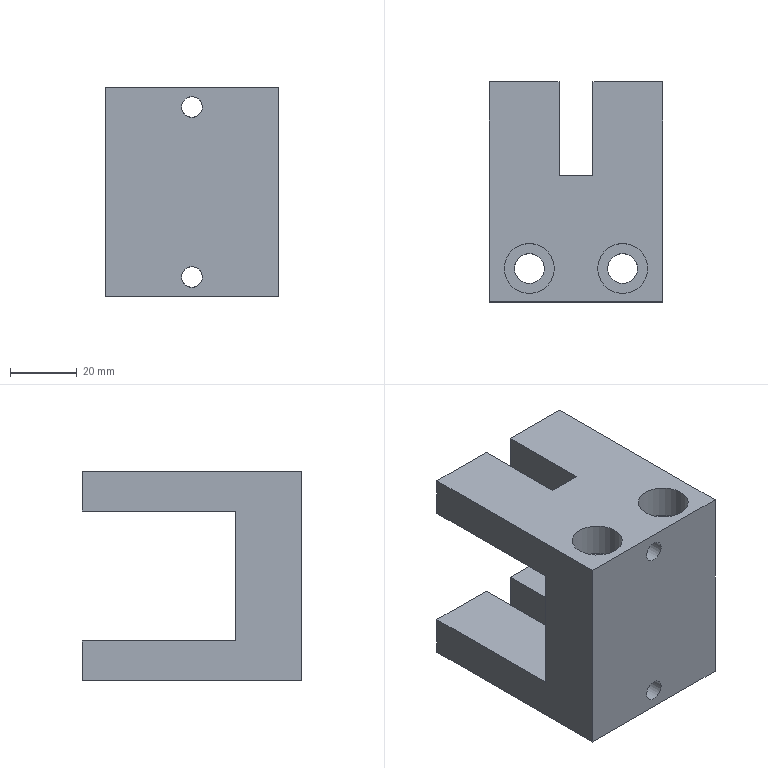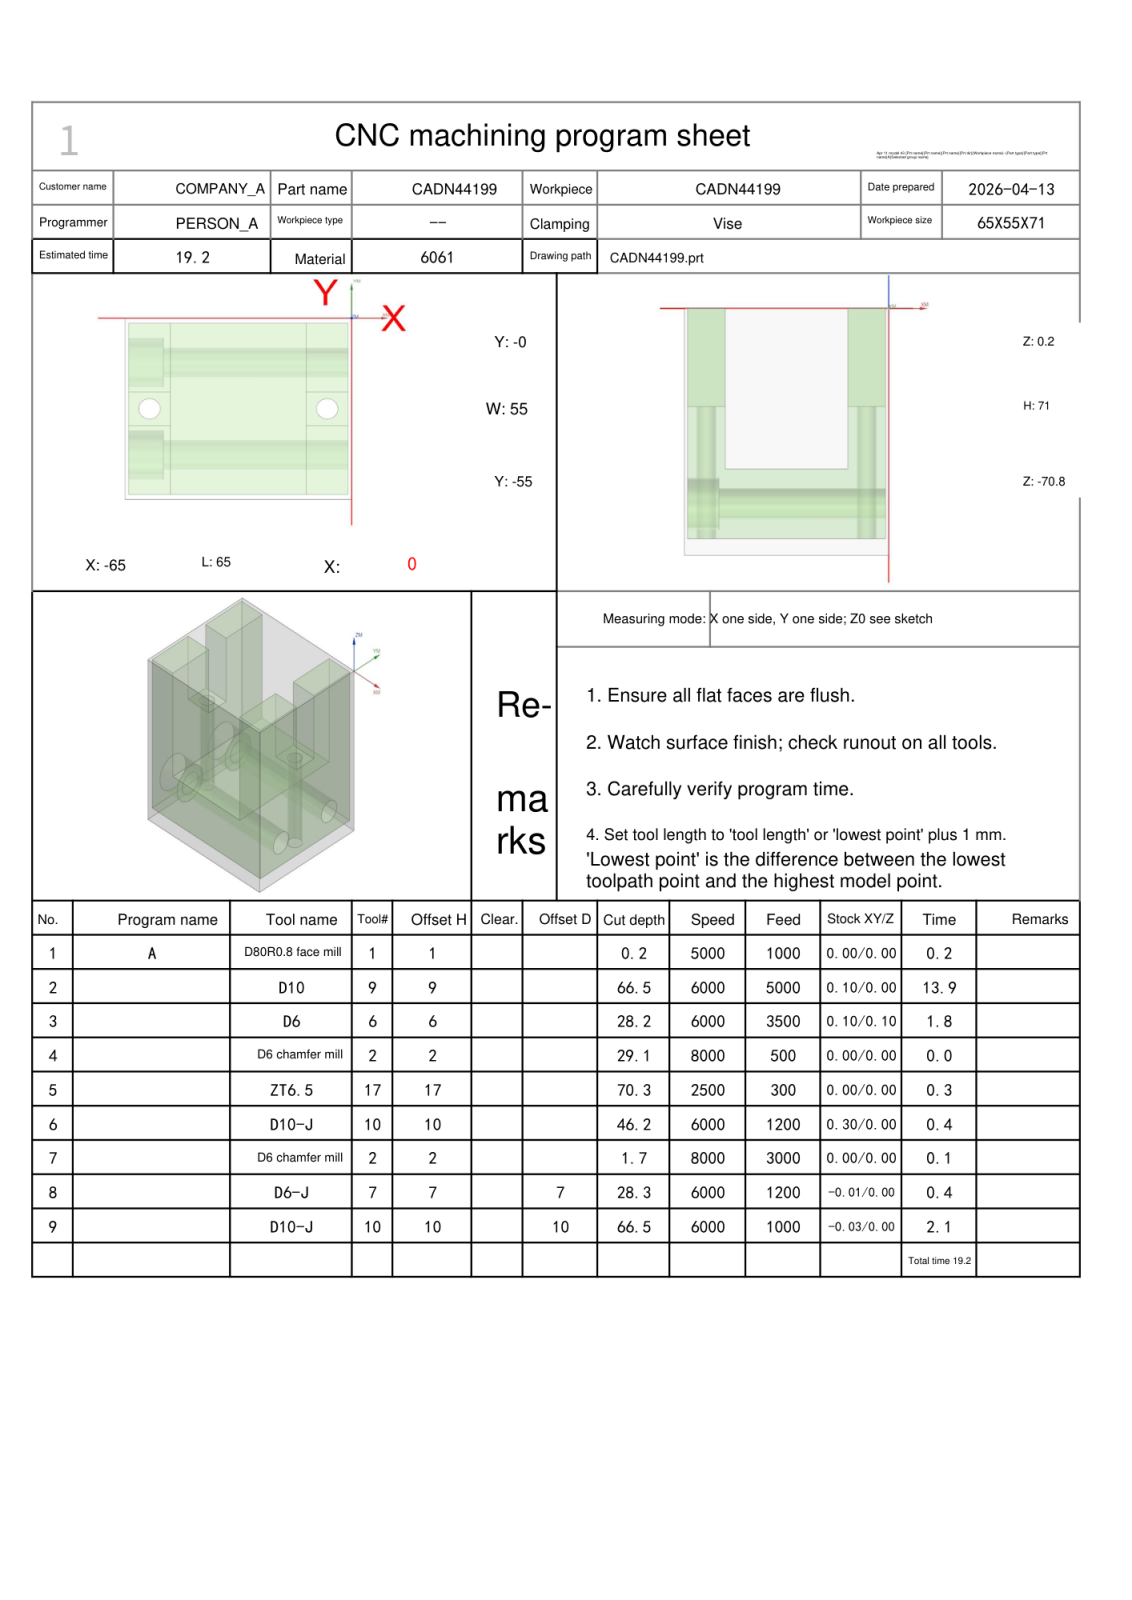NC program | NX | posted by the shop | part box 52 x 66 x 63 mm
Lines 1 to 3030 of 5259, first 2389 of 3028 lines:
%
O0001
(Machine time: 20.73 MIN)
(===Total Tool:7===)
(T1=D80R0.8 face mill D=80.  R=0.8  D-  H01 Z=-0.   )
(T9=D10     D=10.  R=0.   D-  H09 Z=-66.3 )
(T6=D6      D=6.   R=0.   D-  H06 Z=-28.  )
(T2=D6 chamfer mill   D=6.   R=0.   D-  H02 Z=-28.9 )
(T17=ZT6.5  D=6.5  DR_a=118 D-  H17 Z=-70.1 )
(T10=D10-J  D=10.  R=0.   D-  H10 Z=-66.3 )
(T7=D6-J    D=6.   R=0.   D7  H07 Z=-28.1 )
G80 G90 G17 G49 G40
G91 G28 Z0
M01
N1 T01 M06
(D80R0.8 face mill  D=80. R=0.8 H=01 ce=0.00 di=0.00)
G00 G90 G54 X-109. Y-27.5 M03 S5000
G43 H01 Z20.
M08
Z2.
G01 Z0.0 F1000.
X-104.
X39.
X44.
Z2.
G00 Z20.
G91 G28 Z0.0
M05
M09
G91 G28 Z0.0
M01
N2 T09 M06
(D10  D=10. R=0. H=09 ce=0.10 di=0.00)
G00 G90 G54 X-32.5 Y-58.6 M03 S6000
G43 H09 Z20.
M08
Z.5
G01 X-64. Z.404 F5000.
G02 X-69.1 Y-53.5 Z.38 I0.0 J5.1
G01 Y-1.5 Z.222
G02 X-64. Y3.6 Z.198 I5.1 J0.0
G01 X-1. Z.007
G02 X4.1 Y-1.5 Z-.018 I0.0 J-5.1
G01 Y-53.5 Z-.175
G02 X-1. Y-58.6 Z-.2 I-5.1 J0.0
G01 X-64. Z-.391
G02 X-69.1 Y-53.5 Z-.415 I0.0 J5.1
G01 Y-1.5 Z-.573
G02 X-64. Y3.6 Z-.597 I5.1 J0.0
G01 X-1. Z-.788
G02 X4.1 Y-1.5 Z-.813 I0.0 J-5.1
G01 Y-53.5 Z-.971
G02 X-1. Y-58.6 Z-.995 I-5.1 J0.0
G01 X-64. Z-1.186
G02 X-69.1 Y-53.5 Z-1.21 I0.0 J5.1
G01 Y-1.5 Z-1.368
G02 X-64. Y3.6 Z-1.393 I5.1 J0.0
G01 X-1. Z-1.584
G02 X4.1 Y-1.5 Z-1.608 I0.0 J-5.1
G01 Y-53.5 Z-1.766
G02 X-1. Y-58.6 Z-1.79 I-5.1 J0.0
G01 X-64. Z-1.981
G02 X-69.1 Y-53.5 Z-2.006 I0.0 J5.1
G01 Y-1.5 Z-2.163
G02 X-64. Y3.6 Z-2.188 I5.1 J0.0
G01 X-1. Z-2.379
G02 X4.1 Y-1.5 Z-2.403 I0.0 J-5.1
G01 Y-53.5 Z-2.561
G02 X-1. Y-58.6 Z-2.585 I-5.1 J0.0
G01 X-64. Z-2.777
G02 X-69.1 Y-53.5 Z-2.801 I0.0 J5.1
G01 Y-1.5 Z-2.959
G02 X-64. Y3.6 Z-2.983 I5.1 J0.0
G01 X-1. Z-3.174
G02 X4.1 Y-1.5 Z-3.198 I0.0 J-5.1
G01 Y-53.5 Z-3.356
G02 X-1. Y-58.6 Z-3.381 I-5.1 J0.0
G01 X-64. Z-3.572
G02 X-69.1 Y-53.5 Z-3.596 I0.0 J5.1
G01 Y-1.5 Z-3.754
G02 X-64. Y3.6 Z-3.778 I5.1 J0.0
G01 X-1. Z-3.969
G02 X4.1 Y-1.5 Z-3.994 I0.0 J-5.1
G01 Y-53.5 Z-4.152
G02 X-1. Y-58.6 Z-4.176 I-5.1 J0.0
G01 X-64. Z-4.367
G02 X-69.1 Y-53.5 Z-4.391 I0.0 J5.1
G01 Y-1.5 Z-4.549
G02 X-64. Y3.6 Z-4.573 I5.1 J0.0
G01 X-1. Z-4.765
G02 X4.1 Y-1.5 Z-4.789 I0.0 J-5.1
G01 Y-53.5 Z-4.947
G02 X-1. Y-58.6 Z-4.971 I-5.1 J0.0
G01 X-64. Z-5.162
G02 X-69.1 Y-53.5 Z-5.187 I0.0 J5.1
G01 Y-1.5 Z-5.344
G02 X-64. Y3.6 Z-5.369 I5.1 J0.0
G01 X-1. Z-5.56
G02 X4.1 Y-1.5 Z-5.584 I0.0 J-5.1
G01 Y-53.5 Z-5.742
G02 X-1. Y-58.6 Z-5.766 I-5.1 J0.0
G01 X-64. Z-5.958
G02 X-69.1 Y-53.5 Z-5.982 I0.0 J5.1
G01 Y-1.5 Z-6.14
G02 X-64. Y3.6 Z-6.164 I5.1 J0.0
G01 X-1. Z-6.355
G02 X4.1 Y-1.5 Z-6.379 I0.0 J-5.1
G01 Y-53.5 Z-6.537
G02 X-1. Y-58.6 Z-6.562 I-5.1 J0.0
G01 X-64. Z-6.753
G02 X-69.1 Y-53.5 Z-6.777 I0.0 J5.1
G01 Y-1.5 Z-6.935
G02 X-64. Y3.6 Z-6.959 I5.1 J0.0
G01 X-1. Z-7.15
G02 X4.1 Y-1.5 Z-7.175 I0.0 J-5.1
G01 Y-53.5 Z-7.332
G02 X-1. Y-58.6 Z-7.357 I-5.1 J0.0
G01 X-64. Z-7.548
G02 X-69.1 Y-53.5 Z-7.572 I0.0 J5.1
G01 Y-1.5 Z-7.73
G02 X-64. Y3.6 Z-7.754 I5.1 J0.0
G01 X-1. Z-7.946
G02 X4.1 Y-1.5 Z-7.97 I0.0 J-5.1
G01 Y-53.5 Z-8.128
G02 X-1. Y-58.6 Z-8.152 I-5.1 J0.0
G01 X-64. Z-8.343
G02 X-69.1 Y-53.5 Z-8.368 I0.0 J5.1
G01 Y-1.5 Z-8.525
G02 X-64. Y3.6 Z-8.55 I5.1 J0.0
G01 X-1. Z-8.741
G02 X4.1 Y-1.5 Z-8.765 I0.0 J-5.1
G01 Y-53.5 Z-8.923
G02 X-1. Y-58.6 Z-8.947 I-5.1 J0.0
G01 X-64. Z-9.138
G02 X-69.1 Y-53.5 Z-9.163 I0.0 J5.1
G01 Y-1.5 Z-9.321
G02 X-64. Y3.6 Z-9.345 I5.1 J0.0
G01 X-1. Z-9.536
G02 X4.1 Y-1.5 Z-9.56 I0.0 J-5.1
G01 Y-53.5 Z-9.718
G02 X-1. Y-58.6 Z-9.743 I-5.1 J0.0
G01 X-64. Z-9.934
G02 X-69.1 Y-53.5 Z-9.958 I0.0 J5.1
G01 Y-1.5 Z-10.116
G02 X-64. Y3.6 Z-10.14 I5.1 J0.0
G01 X-1. Z-10.331
G02 X4.1 Y-1.5 Z-10.356 I0.0 J-5.1
G01 Y-53.5 Z-10.513
G02 X-1. Y-58.6 Z-10.538 I-5.1 J0.0
G01 X-64. Z-10.729
G02 X-69.1 Y-53.5 Z-10.753 I0.0 J5.1
G01 Y-1.5 Z-10.911
G02 X-64. Y3.6 Z-10.935 I5.1 J0.0
G01 X-1. Z-11.127
G02 X4.1 Y-1.5 Z-11.151 I0.0 J-5.1
G01 Y-53.5 Z-11.309
G02 X-1. Y-58.6 Z-11.333 I-5.1 J0.0
G01 X-64. Z-11.524
G02 X-69.1 Y-53.5 Z-11.548 I0.0 J5.1
G01 Y-1.5 Z-11.706
G02 X-64. Y3.6 Z-11.731 I5.1 J0.0
G01 X-1. Z-11.922
G02 X4.1 Y-1.5 Z-11.946 I0.0 J-5.1
G01 Y-53.5 Z-12.104
G02 X-1. Y-58.6 Z-12.128 I-5.1 J0.0
G01 X-64. Z-12.319
G02 X-69.1 Y-53.5 Z-12.344 I0.0 J5.1
G01 Y-1.5 Z-12.502
G02 X-64. Y3.6 Z-12.526 I5.1 J0.0
G01 X-1. Z-12.717
G02 X4.1 Y-1.5 Z-12.741 I0.0 J-5.1
G01 Y-53.5 Z-12.899
G02 X-1. Y-58.6 Z-12.923 I-5.1 J0.0
G01 X-64. Z-13.115
G02 X-69.1 Y-53.5 Z-13.139 I0.0 J5.1
G01 Y-1.5 Z-13.297
G02 X-64. Y3.6 Z-13.321 I5.1 J0.0
G01 X-1. Z-13.512
G02 X4.1 Y-1.5 Z-13.537 I0.0 J-5.1
G01 Y-53.5 Z-13.694
G02 X-1. Y-58.6 Z-13.719 I-5.1 J0.0
G01 X-64. Z-13.91
G02 X-69.1 Y-53.5 Z-13.934 I0.0 J5.1
G01 Y-1.5 Z-14.092
G02 X-64. Y3.6 Z-14.116 I5.1 J0.0
G01 X-1. Z-14.308
G02 X4.1 Y-1.5 Z-14.332 I0.0 J-5.1
G01 Y-53.5 Z-14.49
G02 X-1. Y-58.6 Z-14.514 I-5.1 J0.0
G01 X-64. Z-14.705
G02 X-69.1 Y-53.5 Z-14.729 I0.0 J5.1
G01 Y-1.5 Z-14.887
G02 X-64. Y3.6 Z-14.912 I5.1 J0.0
G01 X-1. Z-15.103
G02 X4.1 Y-1.5 Z-15.127 I0.0 J-5.1
G01 Y-53.5 Z-15.285
G02 X-1. Y-58.6 Z-15.309 I-5.1 J0.0
G01 X-64. Z-15.5
G02 X-69.1 Y-53.5 Z-15.525 I0.0 J5.1
G01 Y-1.5 Z-15.682
G02 X-64. Y3.6 Z-15.707 I5.1 J0.0
G01 X-1. Z-15.898
G02 X4.1 Y-1.5 Z-15.922 I0.0 J-5.1
G01 Y-53.5 Z-16.08
G02 X-1. Y-58.6 Z-16.104 I-5.1 J0.0
G01 X-64. Z-16.296
G02 X-69.1 Y-53.5 Z-16.32 I0.0 J5.1
G01 Y-1.5 Z-16.478
G02 X-64. Y3.6 Z-16.502 I5.1 J0.0
G01 X-1. Z-16.693
G02 X4.1 Y-1.5 Z-16.718 I0.0 J-5.1
G01 Y-53.5 Z-16.875
G02 X-1. Y-58.6 Z-16.9 I-5.1 J0.0
G01 X-64. Z-17.091
G02 X-69.1 Y-53.5 Z-17.115 I0.0 J5.1
G01 Y-1.5 Z-17.273
G02 X-64. Y3.6 Z-17.297 I5.1 J0.0
G01 X-1. Z-17.488
G02 X4.1 Y-1.5 Z-17.513 I0.0 J-5.1
G01 Y-53.5 Z-17.671
G02 X-1. Y-58.6 Z-17.695 I-5.1 J0.0
G01 X-64. Z-17.886
G02 X-69.1 Y-53.5 Z-17.91 I0.0 J5.1
G01 Y-1.5 Z-18.068
G02 X-64. Y3.6 Z-18.093 I5.1 J0.0
G01 X-1. Z-18.284
G02 X4.1 Y-1.5 Z-18.308 I0.0 J-5.1
G01 Y-53.5 Z-18.466
G02 X-1. Y-58.6 Z-18.49 I-5.1 J0.0
G01 X-64. Z-18.681
G02 X-69.1 Y-53.5 Z-18.706 I0.0 J5.1
G01 Y-1.5 Z-18.863
G02 X-64. Y3.6 Z-18.888 I5.1 J0.0
G01 X-1. Z-19.079
G02 X4.1 Y-1.5 Z-19.103 I0.0 J-5.1
G01 Y-53.5 Z-19.261
G02 X-1. Y-58.6 Z-19.285 I-5.1 J0.0
G01 X-64. Z-19.477
G02 X-69.1 Y-53.5 Z-19.501 I0.0 J5.1
G01 Y-1.5 Z-19.659
G02 X-64. Y3.6 Z-19.683 I5.1 J0.0
G01 X-1. Z-19.874
G02 X4.1 Y-1.5 Z-19.898 I0.0 J-5.1
G01 Y-53.5 Z-20.056
G02 X-1. Y-58.6 Z-20.081 I-5.1 J0.0
G01 X-64. Z-20.272
G02 X-69.1 Y-53.5 Z-20.296 I0.0 J5.1
G01 Y-1.5 Z-20.454
G02 X-64. Y3.6 Z-20.478 I5.1 J0.0
G01 X-1. Z-20.669
G02 X4.1 Y-1.5 Z-20.694 I0.0 J-5.1
G01 Y-53.5 Z-20.852
G02 X-1. Y-58.6 Z-20.876 I-5.1 J0.0
G01 X-64. Z-21.067
G02 X-69.1 Y-53.5 Z-21.091 I0.0 J5.1
G01 Y-1.5 Z-21.249
G02 X-64. Y3.6 Z-21.273 I5.1 J0.0
G01 X-1. Z-21.465
G02 X4.1 Y-1.5 Z-21.489 I0.0 J-5.1
G01 Y-53.5 Z-21.647
G02 X-1. Y-58.6 Z-21.671 I-5.1 J0.0
G01 X-64. Z-21.862
G02 X-69.1 Y-53.5 Z-21.887 I0.0 J5.1
G01 Y-1.5 Z-22.044
G02 X-64. Y3.6 Z-22.069 I5.1 J0.0
G01 X-1. Z-22.26
G02 X4.1 Y-1.5 Z-22.284 I0.0 J-5.1
G01 Y-53.5 Z-22.442
G02 X-1. Y-58.6 Z-22.466 I-5.1 J0.0
G01 X-64. Z-22.658
G02 X-69.1 Y-53.5 Z-22.682 I0.0 J5.1
G01 Y-1.5 Z-22.84
G02 X-64. Y3.6 Z-22.864 I5.1 J0.0
G01 X-1. Z-23.055
G02 X4.1 Y-1.5 Z-23.079 I0.0 J-5.1
G01 Y-53.5 Z-23.237
G02 X-1. Y-58.6 Z-23.262 I-5.1 J0.0
G01 X-64. Z-23.453
G02 X-69.1 Y-53.5 Z-23.477 I0.0 J5.1
G01 Y-1.5 Z-23.635
G02 X-64. Y3.6 Z-23.659 I5.1 J0.0
G01 X-1. Z-23.85
G02 X4.1 Y-1.5 Z-23.875 I0.0 J-5.1
G01 Y-53.5 Z-24.032
G02 X-1. Y-58.6 Z-24.057 I-5.1 J0.0
G01 X-64. Z-24.248
G02 X-69.1 Y-53.5 Z-24.272 I0.0 J5.1
G01 Y-1.5 Z-24.43
G02 X-64. Y3.6 Z-24.454 I5.1 J0.0
G01 X-1. Z-24.646
G02 X4.1 Y-1.5 Z-24.67 I0.0 J-5.1
G01 Y-53.5 Z-24.828
G02 X-1. Y-58.6 Z-24.852 I-5.1 J0.0
G01 X-64. Z-25.043
G02 X-69.1 Y-53.5 Z-25.068 I0.0 J5.1
G01 Y-1.5 Z-25.225
G02 X-64. Y3.6 Z-25.25 I5.1 J0.0
G01 X-1. Z-25.441
G02 X4.1 Y-1.5 Z-25.465 I0.0 J-5.1
G01 Y-53.5 Z-25.623
G02 X-1. Y-58.6 Z-25.647 I-5.1 J0.0
G01 X-64. Z-25.838
G02 X-69.1 Y-53.5 Z-25.863 I0.0 J5.1
G01 Y-1.5 Z-26.021
G02 X-64. Y3.6 Z-26.045 I5.1 J0.0
G01 X-1. Z-26.236
G02 X4.1 Y-1.5 Z-26.26 I0.0 J-5.1
G01 Y-53.5 Z-26.418
G02 X-1. Y-58.6 Z-26.443 I-5.1 J0.0
G01 X-64. Z-26.634
G02 X-69.1 Y-53.5 Z-26.658 I0.0 J5.1
G01 Y-1.5 Z-26.816
G02 X-64. Y3.6 Z-26.84 I5.1 J0.0
G01 X-1. Z-27.031
G02 X4.1 Y-1.5 Z-27.056 I0.0 J-5.1
G01 Y-53.5 Z-27.213
G02 X-1. Y-58.6 Z-27.238 I-5.1 J0.0
G01 X-64. Z-27.429
G02 X-69.1 Y-53.5 Z-27.453 I0.0 J5.1
G01 Y-1.5 Z-27.611
G02 X-64. Y3.6 Z-27.635 I5.1 J0.0
G01 X-1. Z-27.827
G02 X4.1 Y-1.5 Z-27.851 I0.0 J-5.1
G01 Y-53.5 Z-28.009
G02 X-1. Y-58.6 Z-28.033 I-5.1 J0.0
G01 X-64. Z-28.224
G02 X-69.1 Y-53.5 Z-28.248 I0.0 J5.1
G01 Y-1.5 Z-28.406
G02 X-64. Y3.6 Z-28.431 I5.1 J0.0
G01 X-1. Z-28.622
G02 X4.1 Y-1.5 Z-28.646 I0.0 J-5.1
G01 Y-53.5 Z-28.804
G02 X-1. Y-58.6 Z-28.828 I-5.1 J0.0
G01 X-64. Z-29.019
G02 X-69.1 Y-53.5 Z-29.044 I0.0 J5.1
G01 Y-1.5 Z-29.202
G02 X-64. Y3.6 Z-29.226 I5.1 J0.0
G01 X-1. Z-29.417
G02 X4.1 Y-1.5 Z-29.441 I0.0 J-5.1
G01 Y-53.5 Z-29.599
G02 X-1. Y-58.6 Z-29.623 I-5.1 J0.0
G01 X-64. Z-29.815
G02 X-69.1 Y-53.5 Z-29.839 I0.0 J5.1
G01 Y-1.5 Z-29.997
G02 X-64. Y3.6 Z-30.021 I5.1 J0.0
G01 X-1. Z-30.212
G02 X4.1 Y-1.5 Z-30.237 I0.0 J-5.1
G01 Y-53.5 Z-30.394
G02 X-1. Y-58.6 Z-30.419 I-5.1 J0.0
G01 X-64. Z-30.61
G02 X-69.1 Y-53.5 Z-30.634 I0.0 J5.1
G01 Y-1.5 Z-30.792
G02 X-64. Y3.6 Z-30.816 I5.1 J0.0
G01 X-1. Z-31.008
G02 X4.1 Y-1.5 Z-31.032 I0.0 J-5.1
G01 Y-53.5 Z-31.19
G02 X-1. Y-58.6 Z-31.214 I-5.1 J0.0
G01 X-64. Z-31.405
G02 X-69.1 Y-53.5 Z-31.429 I0.0 J5.1
G01 Y-1.5 Z-31.587
G02 X-64. Y3.6 Z-31.612 I5.1 J0.0
G01 X-1. Z-31.803
G02 X4.1 Y-1.5 Z-31.827 I0.0 J-5.1
G01 Y-53.5 Z-31.985
G02 X-1. Y-58.6 Z-32.009 I-5.1 J0.0
G01 X-64. Z-32.2
G02 X-69.1 Y-53.5 Z-32.225 I0.0 J5.1
G01 Y-1.5 Z-32.382
G02 X-64. Y3.6 Z-32.407 I5.1 J0.0
G01 X-1. Z-32.598
G02 X4.1 Y-1.5 Z-32.622 I0.0 J-5.1
G01 Y-53.5 Z-32.78
G02 X-1. Y-58.6 Z-32.804 I-5.1 J0.0
G01 X-64. Z-32.996
G02 X-69.1 Y-53.5 Z-33.02 I0.0 J5.1
G01 Y-1.5 Z-33.178
G02 X-64. Y3.6 Z-33.202 I5.1 J0.0
G01 X-1. Z-33.393
G02 X4.1 Y-1.5 Z-33.418 I0.0 J-5.1
G01 Y-53.5 Z-33.575
G02 X-1. Y-58.6 Z-33.6 I-5.1 J0.0
G01 X-64. Z-33.791
G02 X-69.1 Y-53.5 Z-33.815 I0.0 J5.1
G01 Y-1.5 Z-33.973
G02 X-64. Y3.6 Z-33.997 I5.1 J0.0
G01 X-1. Z-34.188
G02 X4.1 Y-1.5 Z-34.213 I0.0 J-5.1
G01 Y-53.5 Z-34.371
G02 X-1. Y-58.6 Z-34.395 I-5.1 J0.0
G01 X-64. Z-34.586
G02 X-69.1 Y-53.5 Z-34.61 I0.0 J5.1
G01 Y-1.5 Z-34.768
G02 X-64. Y3.6 Z-34.793 I5.1 J0.0
G01 X-1. Z-34.984
G02 X4.1 Y-1.5 Z-35.008 I0.0 J-5.1
G01 Y-53.5 Z-35.166
G02 X-1. Y-58.6 Z-35.19 I-5.1 J0.0
G01 X-64. Z-35.381
G02 X-69.1 Y-53.5 Z-35.406 I0.0 J5.1
G01 Y-1.5 Z-35.563
G02 X-64. Y3.6 Z-35.588 I5.1 J0.0
G01 X-1. Z-35.779
G02 X4.1 Y-1.5 Z-35.803 I0.0 J-5.1
G01 Y-53.5 Z-35.961
G02 X-1. Y-58.6 Z-35.985 I-5.1 J0.0
G01 X-64. Z-36.177
G02 X-69.1 Y-53.5 Z-36.201 I0.0 J5.1
G01 Y-1.5 Z-36.359
G02 X-64. Y3.6 Z-36.383 I5.1 J0.0
G01 X-1. Z-36.574
G02 X4.1 Y-1.5 Z-36.598 I0.0 J-5.1
G01 Y-53.5 Z-36.756
G02 X-1. Y-58.6 Z-36.781 I-5.1 J0.0
G01 X-64. Z-36.972
G02 X-69.1 Y-53.5 Z-36.996 I0.0 J5.1
G01 Y-1.5 Z-37.154
G02 X-64. Y3.6 Z-37.178 I5.1 J0.0
G01 X-1. Z-37.369
G02 X4.1 Y-1.5 Z-37.394 I0.0 J-5.1
G01 Y-53.5 Z-37.552
G02 X-1. Y-58.6 Z-37.576 I-5.1 J0.0
G01 X-64. Z-37.767
G02 X-69.1 Y-53.5 Z-37.791 I0.0 J5.1
G01 Y-1.5 Z-37.949
G02 X-64. Y3.6 Z-37.973 I5.1 J0.0
G01 X-1. Z-38.165
G02 X4.1 Y-1.5 Z-38.189 I0.0 J-5.1
G01 Y-53.5 Z-38.347
G02 X-1. Y-58.6 Z-38.371 I-5.1 J0.0
G01 X-64. Z-38.562
G02 X-69.1 Y-53.5 Z-38.587 I0.0 J5.1
G01 Y-1.5 Z-38.744
G02 X-64. Y3.6 Z-38.769 I5.1 J0.0
G01 X-1. Z-38.96
G02 X4.1 Y-1.5 Z-38.984 I0.0 J-5.1
G01 Y-53.5 Z-39.142
G02 X-1. Y-58.6 Z-39.166 I-5.1 J0.0
G01 X-64. Z-39.358
G02 X-69.1 Y-53.5 Z-39.382 I0.0 J5.1
G01 Y-1.5 Z-39.54
G02 X-64. Y3.6 Z-39.564 I5.1 J0.0
G01 X-1. Z-39.755
G02 X4.1 Y-1.5 Z-39.779 I0.0 J-5.1
G01 Y-53.5 Z-39.937
G02 X-1. Y-58.6 Z-39.962 I-5.1 J0.0
G01 X-64. Z-40.153
G02 X-69.1 Y-53.5 Z-40.177 I0.0 J5.1
G01 Y-1.5 Z-40.335
G02 X-64. Y3.6 Z-40.359 I5.1 J0.0
G01 X-1. Z-40.55
G02 X4.1 Y-1.5 Z-40.575 I0.0 J-5.1
G01 Y-53.5 Z-40.732
G02 X-1. Y-58.6 Z-40.757 I-5.1 J0.0
G01 X-64. Z-40.948
G02 X-69.1 Y-53.5 Z-40.972 I0.0 J5.1
G01 Y-1.5 Z-41.13
G02 X-64. Y3.6 Z-41.154 I5.1 J0.0
G01 X-1. Z-41.346
G02 X4.1 Y-1.5 Z-41.37 I0.0 J-5.1
G01 Y-53.5 Z-41.528
G02 X-1. Y-58.6 Z-41.552 I-5.1 J0.0
G01 X-64. Z-41.743
G02 X-69.1 Y-53.5 Z-41.768 I0.0 J5.1
G01 Y-1.5 Z-41.925
G02 X-64. Y3.6 Z-41.95 I5.1 J0.0
G01 X-1. Z-42.141
G02 X4.1 Y-1.5 Z-42.165 I0.0 J-5.1
G01 Y-53.5 Z-42.323
G02 X-1. Y-58.6 Z-42.347 I-5.1 J0.0
G01 X-64. Z-42.538
G02 X-69.1 Y-53.5 Z-42.563 I0.0 J5.1
G01 Y-1.5 Z-42.721
G02 X-64. Y3.6 Z-42.745 I5.1 J0.0
G01 X-1. Z-42.936
G02 X4.1 Y-1.5 Z-42.96 I0.0 J-5.1
G01 Y-53.5 Z-43.118
G02 X-1. Y-58.6 Z-43.143 I-5.1 J0.0
G01 X-64. Z-43.334
G02 X-69.1 Y-53.5 Z-43.358 I0.0 J5.1
G01 Y-1.5 Z-43.516
G02 X-64. Y3.6 Z-43.54 I5.1 J0.0
G01 X-1. Z-43.731
G02 X4.1 Y-1.5 Z-43.756 I0.0 J-5.1
G01 Y-53.5 Z-43.913
G02 X-1. Y-58.6 Z-43.938 I-5.1 J0.0
G01 X-64. Z-44.129
G02 X-69.1 Y-53.5 Z-44.153 I0.0 J5.1
G01 Y-1.5 Z-44.311
G02 X-64. Y3.6 Z-44.335 I5.1 J0.0
G01 X-1. Z-44.527
G02 X4.1 Y-1.5 Z-44.551 I0.0 J-5.1
G01 Y-53.5 Z-44.709
G02 X-1. Y-58.6 Z-44.733 I-5.1 J0.0
G01 X-64. Z-44.924
G02 X-69.1 Y-53.5 Z-44.948 I0.0 J5.1
G01 Y-1.5 Z-45.106
G02 X-64. Y3.6 Z-45.131 I5.1 J0.0
G01 X-1. Z-45.322
G02 X4.1 Y-1.5 Z-45.346 I0.0 J-5.1
G01 Y-53.5 Z-45.504
G02 X-1. Y-58.6 Z-45.528 I-5.1 J0.0
G01 X-64. Z-45.719
G02 X-69.1 Y-53.5 Z-45.744 I0.0 J5.1
G01 Y-1.5 Z-45.902
G02 X-64. Y3.6 Z-45.926 I5.1 J0.0
G01 X-1. Z-46.117
G02 X4.1 Y-1.5 Z-46.141 I0.0 J-5.1
G01 Y-53.5 Z-46.299
G02 X-1. Y-58.6 Z-46.323 I-5.1 J0.0
G01 X-64. Z-46.515
G02 X-69.1 Y-53.5 Z-46.539 I0.0 J5.1
G01 Y-1.5 Z-46.697
G02 X-64. Y3.6 Z-46.721 I5.1 J0.0
G01 X-1. Z-46.912
G02 X4.1 Y-1.5 Z-46.937 I0.0 J-5.1
G01 Y-53.5 Z-47.094
G02 X-1. Y-58.6 Z-47.119 I-5.1 J0.0
G01 X-64. Z-47.31
G02 X-69.1 Y-53.5 Z-47.334 I0.0 J5.1
G01 Y-1.5 Z-47.492
G02 X-64. Y3.6 Z-47.516 I5.1 J0.0
G01 X-1. Z-47.708
G02 X4.1 Y-1.5 Z-47.732 I0.0 J-5.1
G01 Y-53.5 Z-47.89
G02 X-1. Y-58.6 Z-47.914 I-5.1 J0.0
G01 X-64. Z-48.105
G02 X-69.1 Y-53.5 Z-48.129 I0.0 J5.1
G01 Y-1.5 Z-48.287
G02 X-64. Y3.6 Z-48.312 I5.1 J0.0
G01 X-1. Z-48.503
G02 X4.1 Y-1.5 Z-48.527 I0.0 J-5.1
G01 Y-53.5 Z-48.685
G02 X-1. Y-58.6 Z-48.709 I-5.1 J0.0
G01 X-64. Z-48.9
G02 X-69.1 Y-53.5 Z-48.925 I0.0 J5.1
G01 Y-1.5 Z-49.082
G02 X-64. Y3.6 Z-49.107 I5.1 J0.0
G01 X-1. Z-49.298
G02 X4.1 Y-1.5 Z-49.322 I0.0 J-5.1
G01 Y-53.5 Z-49.48
G02 X-1. Y-58.6 Z-49.504 I-5.1 J0.0
G01 X-64. Z-49.696
G02 X-69.1 Y-53.5 Z-49.72 I0.0 J5.1
G01 Y-1.5 Z-49.878
G02 X-64. Y3.6 Z-49.902 I5.1 J0.0
G01 X-1. Z-50.093
G02 X4.1 Y-1.5 Z-50.118 I0.0 J-5.1
G01 Y-53.5 Z-50.275
G02 X-1. Y-58.6 Z-50.3 I-5.1 J0.0
G01 X-64. Z-50.491
G02 X-69.1 Y-53.5 Z-50.515 I0.0 J5.1
G01 Y-1.5 Z-50.673
G02 X-64. Y3.6 Z-50.697 I5.1 J0.0
G01 X-1. Z-50.888
G02 X4.1 Y-1.5 Z-50.913 I0.0 J-5.1
G01 Y-53.5 Z-51.071
G02 X-1. Y-58.6 Z-51.095 I-5.1 J0.0
G01 X-64. Z-51.286
G02 X-69.1 Y-53.5 Z-51.31 I0.0 J5.1
G01 Y-1.5 Z-51.468
G02 X-64. Y3.6 Z-51.493 I5.1 J0.0
G01 X-1. Z-51.684
G02 X4.1 Y-1.5 Z-51.708 I0.0 J-5.1
G01 Y-53.5 Z-51.866
G02 X-1. Y-58.6 Z-51.89 I-5.1 J0.0
G01 X-64. Z-52.081
G02 X-69.1 Y-53.5 Z-52.106 I0.0 J5.1
G01 Y-1.5 Z-52.263
G02 X-64. Y3.6 Z-52.288 I5.1 J0.0
G01 X-1. Z-52.479
G02 X4.1 Y-1.5 Z-52.503 I0.0 J-5.1
G01 Y-53.5 Z-52.661
G02 X-1. Y-58.6 Z-52.685 I-5.1 J0.0
G01 X-64. Z-52.877
G02 X-69.1 Y-53.5 Z-52.901 I0.0 J5.1
G01 Y-1.5 Z-53.059
G02 X-64. Y3.6 Z-53.083 I5.1 J0.0
G01 X-1. Z-53.274
G02 X4.1 Y-1.5 Z-53.298 I0.0 J-5.1
G01 Y-53.5 Z-53.456
G02 X-1. Y-58.6 Z-53.481 I-5.1 J0.0
G01 X-64. Z-53.672
G02 X-69.1 Y-53.5 Z-53.696 I0.0 J5.1
G01 Y-1.5 Z-53.854
G02 X-64. Y3.6 Z-53.878 I5.1 J0.0
G01 X-1. Z-54.069
G02 X4.1 Y-1.5 Z-54.094 I0.0 J-5.1
G01 Y-53.5 Z-54.252
G02 X-1. Y-58.6 Z-54.276 I-5.1 J0.0
G01 X-64. Z-54.467
G02 X-69.1 Y-53.5 Z-54.491 I0.0 J5.1
G01 Y-1.5 Z-54.649
G02 X-64. Y3.6 Z-54.673 I5.1 J0.0
G01 X-1. Z-54.865
G02 X4.1 Y-1.5 Z-54.889 I0.0 J-5.1
G01 Y-53.5 Z-55.047
G02 X-1. Y-58.6 Z-55.071 I-5.1 J0.0
G01 X-64. Z-55.262
G02 X-69.1 Y-53.5 Z-55.287 I0.0 J5.1
G01 Y-1.5 Z-55.444
G02 X-64. Y3.6 Z-55.469 I5.1 J0.0
G01 X-1. Z-55.66
G02 X4.1 Y-1.5 Z-55.684 I0.0 J-5.1
G01 Y-53.5 Z-55.842
G02 X-1. Y-58.6 Z-55.866 I-5.1 J0.0
G01 X-64. Z-56.058
G02 X-69.1 Y-53.5 Z-56.082 I0.0 J5.1
G01 Y-1.5 Z-56.24
G02 X-64. Y3.6 Z-56.264 I5.1 J0.0
G01 X-1. Z-56.455
G02 X4.1 Y-1.5 Z-56.479 I0.0 J-5.1
G01 Y-53.5 Z-56.637
G02 X-1. Y-58.6 Z-56.662 I-5.1 J0.0
G01 X-64. Z-56.853
G02 X-69.1 Y-53.5 Z-56.877 I0.0 J5.1
G01 Y-1.5 Z-57.035
G02 X-64. Y3.6 Z-57.059 I5.1 J0.0
G01 X-1. Z-57.25
G02 X4.1 Y-1.5 Z-57.275 I0.0 J-5.1
G01 Y-53.5 Z-57.432
G02 X-1. Y-58.6 Z-57.457 I-5.1 J0.0
G01 X-64. Z-57.648
G02 X-69.1 Y-53.5 Z-57.672 I0.0 J5.1
G01 Y-1.5 Z-57.83
G02 X-64. Y3.6 Z-57.854 I5.1 J0.0
G01 X-1. Z-58.046
G02 X4.1 Y-1.5 Z-58.07 I0.0 J-5.1
G01 Y-53.5 Z-58.228
G02 X-1. Y-58.6 Z-58.252 I-5.1 J0.0
G01 X-64. Z-58.443
G02 X-69.1 Y-53.5 Z-58.468 I0.0 J5.1
G01 Y-1.5 Z-58.625
G02 X-64. Y3.6 Z-58.65 I5.1 J0.0
G01 X-1. Z-58.841
G02 X4.1 Y-1.5 Z-58.865 I0.0 J-5.1
G01 Y-53.5 Z-59.023
G02 X-1. Y-58.6 Z-59.047 I-5.1 J0.0
G01 X-64. Z-59.238
G02 X-69.1 Y-53.5 Z-59.263 I0.0 J5.1
G01 Y-1.5 Z-59.421
G02 X-64. Y3.6 Z-59.445 I5.1 J0.0
G01 X-1. Z-59.636
G02 X4.1 Y-1.5 Z-59.66 I0.0 J-5.1
G01 Y-53.5 Z-59.818
G02 X-1. Y-58.6 Z-59.843 I-5.1 J0.0
G01 X-64. Z-60.034
G02 X-69.1 Y-53.5 Z-60.058 I0.0 J5.1
G01 Y-1.5 Z-60.216
G02 X-64. Y3.6 Z-60.24 I5.1 J0.0
G01 X-1. Z-60.431
G02 X4.1 Y-1.5 Z-60.456 I0.0 J-5.1
G01 Y-53.5 Z-60.613
G02 X-1. Y-58.6 Z-60.638 I-5.1 J0.0
G01 X-64. Z-60.829
G02 X-69.1 Y-53.5 Z-60.853 I0.0 J5.1
G01 Y-1.5 Z-61.011
G02 X-64. Y3.6 Z-61.035 I5.1 J0.0
G01 X-1. Z-61.227
G02 X4.1 Y-1.5 Z-61.251 I0.0 J-5.1
G01 Y-53.5 Z-61.409
G02 X-1. Y-58.6 Z-61.433 I-5.1 J0.0
G01 X-64. Z-61.624
G02 X-69.1 Y-53.5 Z-61.648 I0.0 J5.1
G01 Y-1.5 Z-61.806
G02 X-64. Y3.6 Z-61.831 I5.1 J0.0
G01 X-1. Z-62.022
G02 X4.1 Y-1.5 Z-62.046 I0.0 J-5.1
G01 Y-53.5 Z-62.204
G02 X-1. Y-58.6 Z-62.228 I-5.1 J0.0
G01 X-64. Z-62.419
G02 X-69.1 Y-53.5 Z-62.444 I0.0 J5.1
G01 Y-1.5 Z-62.602
G02 X-64. Y3.6 Z-62.626 I5.1 J0.0
G01 X-1. Z-62.817
G02 X4.1 Y-1.5 Z-62.841 I0.0 J-5.1
G01 Y-53.5 Z-62.999
G02 X-1. Y-58.6 Z-63.023 I-5.1 J0.0
G01 X-64. Z-63.215
G02 X-69.1 Y-53.5 Z-63.239 I0.0 J5.1
G01 Y-1.5 Z-63.397
G02 X-64. Y3.6 Z-63.421 I5.1 J0.0
G01 X-1. Z-63.612
G02 X4.1 Y-1.5 Z-63.637 I0.0 J-5.1
G01 Y-53.5 Z-63.794
G02 X-1. Y-58.6 Z-63.819 I-5.1 J0.0
G01 X-64. Z-64.01
G02 X-69.1 Y-53.5 Z-64.034 I0.0 J5.1
G01 Y-1.5 Z-64.192
G02 X-64. Y3.6 Z-64.216 I5.1 J0.0
G01 X-1. Z-64.408
G02 X4.1 Y-1.5 Z-64.432 I0.0 J-5.1
G01 Y-53.5 Z-64.59
G02 X-1. Y-58.6 Z-64.614 I-5.1 J0.0
G01 X-64. Z-64.805
G02 X-69.1 Y-53.5 Z-64.829 I0.0 J5.1
G01 Y-1.5 Z-64.987
G02 X-64. Y3.6 Z-65.012 I5.1 J0.0
G01 X-1. Z-65.203
G02 X4.1 Y-1.5 Z-65.227 I0.0 J-5.1
G01 Y-53.5 Z-65.385
G02 X-1. Y-58.6 Z-65.409 I-5.1 J0.0
G01 X-64. Z-65.6
G02 X-69.1 Y-53.5 Z-65.625 I0.0 J5.1
G01 Y-1.5 Z-65.782
G02 X-64. Y3.6 Z-65.807 I5.1 J0.0
G01 X-1. Z-65.998
G02 X4.1 Y-1.5 Z-66.022 I0.0 J-5.1
G01 Y-53.5 Z-66.18
G02 X-1. Y-58.6 Z-66.204 I-5.1 J0.0
G01 X-32.5 Z-66.3
X-64.
G02 X-69.1 Y-53.5 I0.0 J5.1
G01 Y-1.5
G02 X-64. Y3.6 I5.1 J0.0
G01 X-1.
G02 X4.1 Y-1.5 I0.0 J-5.1
G01 Y-53.5
G02 X-1. Y-58.6 I-5.1 J0.0
G01 X-32.5
X-33.
Z-65.3
G00 Z20.
G00 G90 X-32.5 Y-61.5 M03 S6000
Z20.
Z.001
G01 Z-.499 F3500.
Y-54.5
X-46.9
Y-.5
X-18.1
Y-54.5
X-32.5
Y-47.5
X-39.9
Y-7.5
X-25.1
Y-47.5
X-32.5
Y-40.5
X-32.9
Y-14.5
X-32.1
Y-40.5
X-32.5
X-32.9
Y-40.4
Z.001
G00 Z.5
X-32.5 Y-61.5
Z-.498
G01 Z-.998
Y-54.5
X-46.9
Y-.5
X-18.1
Y-54.5
X-32.5
Y-47.5
X-39.9
Y-7.5
X-25.1
Y-47.5
X-32.5
Y-40.5
X-32.9
Y-14.5
X-32.1
Y-40.5
X-32.5
X-32.9
Y-40.4
Z-.498
G00 Z.001
X-32.5 Y-61.5
Z-.997
G01 Z-1.497
Y-54.5
X-46.9
Y-.5
X-18.1
Y-54.5
X-32.5
Y-47.5
X-39.9
Y-7.5
X-25.1
Y-47.5
X-32.5
Y-40.5
X-32.9
Y-14.5
X-32.1
Y-40.5
X-32.5
X-32.9
Y-40.4
Z-.997
G00 Z-.498
X-32.5 Y-61.5
Z-1.496
G01 Z-1.996
Y-54.5
X-46.9
Y-.5
X-18.1
Y-54.5
X-32.5
Y-47.5
X-39.9
Y-7.5
X-25.1
Y-47.5
X-32.5
Y-40.5
X-32.9
Y-14.5
X-32.1
Y-40.5
X-32.5
X-32.9
Y-40.4
Z-1.496
G00 Z-.997
X-32.5 Y-61.5
Z-1.995
G01 Z-2.495
Y-54.5
X-46.9
Y-.5
X-18.1
Y-54.5
X-32.5
Y-47.5
X-39.9
Y-7.5
X-25.1
Y-47.5
X-32.5
Y-40.5
X-32.9
Y-14.5
X-32.1
Y-40.5
X-32.5
X-32.9
Y-40.4
Z-1.995
G00 Z-1.496
X-32.5 Y-61.5
Z-2.493
G01 Z-2.993
Y-54.5
X-46.9
Y-.5
X-18.1
Y-54.5
X-32.5
Y-47.5
X-39.9
Y-7.5
X-25.1
Y-47.5
X-32.5
Y-40.5
X-32.9
Y-14.5
X-32.1
Y-40.5
X-32.5
X-32.9
Y-40.4
Z-2.493
G00 Z-1.995
X-32.5 Y-61.5
Z-2.992
G01 Z-3.492
Y-54.5
X-46.9
Y-.5
X-18.1
Y-54.5
X-32.5
Y-47.5
X-39.9
Y-7.5
X-25.1
Y-47.5
X-32.5
Y-40.5
X-32.9
Y-14.5
X-32.1
Y-40.5
X-32.5
X-32.9
Y-40.4
Z-2.992
G00 Z-2.493
X-32.5 Y-61.5
Z-3.491
G01 Z-3.991
Y-54.5
X-46.9
Y-.5
X-18.1
Y-54.5
X-32.5
Y-47.5
X-39.9
Y-7.5
X-25.1
Y-47.5
X-32.5
Y-40.5
X-32.9
Y-14.5
X-32.1
Y-40.5
X-32.5
X-32.9
Y-40.4
Z-3.491
G00 Z-2.992
X-32.5 Y-61.5
Z-3.99
G01 Z-4.49
Y-54.5
X-46.9
Y-.5
X-18.1
Y-54.5
X-32.5
Y-47.5
X-39.9
Y-7.5
X-25.1
Y-47.5
X-32.5
Y-40.5
X-32.9
Y-14.5
X-32.1
Y-40.5
X-32.5
X-32.9
Y-40.4
Z-3.99
G00 Z-3.491
X-32.5 Y-61.5
Z-4.489
G01 Z-4.989
Y-54.5
X-46.9
Y-.5
X-18.1
Y-54.5
X-32.5
Y-47.5
X-39.9
Y-7.5
X-25.1
Y-47.5
X-32.5
Y-40.5
X-32.9
Y-14.5
X-32.1
Y-40.5
X-32.5
X-32.9
Y-40.4
Z-4.489
G00 Z-3.99
X-32.5 Y-61.5
Z-4.988
G01 Z-5.488
Y-54.5
X-46.9
Y-.5
X-18.1
Y-54.5
X-32.5
Y-47.5
X-39.9
Y-7.5
X-25.1
Y-47.5
X-32.5
Y-40.5
X-32.9
Y-14.5
X-32.1
Y-40.5
X-32.5
X-32.9
Y-40.4
Z-4.988
G00 Z-4.489
X-32.5 Y-61.5
Z-5.487
G01 Z-5.987
Y-54.5
X-46.9
Y-.5
X-18.1
Y-54.5
X-32.5
Y-47.5
X-39.9
Y-7.5
X-25.1
Y-47.5
X-32.5
Y-40.5
X-32.9
Y-14.5
X-32.1
Y-40.5
X-32.5
X-32.9
Y-40.4
Z-5.487
G00 Z-4.988
X-32.5 Y-61.5
Z-5.986
G01 Z-6.486
Y-54.5
X-46.9
Y-.5
X-18.1
Y-54.5
X-32.5
Y-47.5
X-39.9
Y-7.5
X-25.1
Y-47.5
X-32.5
Y-40.5
X-32.9
Y-14.5
X-32.1
Y-40.5
X-32.5
X-32.9
Y-40.4
Z-5.986
G00 Z-5.487
X-32.5 Y-61.5
Z-6.485
G01 Z-6.985
Y-54.5
X-46.9
Y-.5
X-18.1
Y-54.5
X-32.5
Y-47.5
X-39.9
Y-7.5
X-25.1
Y-47.5
X-32.5
Y-40.5
X-32.9
Y-14.5
X-32.1
Y-40.5
X-32.5
X-32.9
Y-40.4
Z-6.485
G00 Z-5.986
X-32.5 Y-61.5
Z-6.984
G01 Z-7.484
Y-54.5
X-46.9
Y-.5
X-18.1
Y-54.5
X-32.5
Y-47.5
X-39.9
Y-7.5
X-25.1
Y-47.5
X-32.5
Y-40.5
X-32.9
Y-14.5
X-32.1
Y-40.5
X-32.5
X-32.9
Y-40.4
Z-6.984
G00 Z-6.485
X-32.5 Y-61.5
Z-7.483
G01 Z-7.983
Y-54.5
X-46.9
Y-.5
X-18.1
Y-54.5
X-32.5
Y-47.5
X-39.9
Y-7.5
X-25.1
Y-47.5
X-32.5
Y-40.5
X-32.9
Y-14.5
X-32.1
Y-40.5
X-32.5
X-32.9
Y-40.4
Z-7.483
G00 Z-6.984
X-32.5 Y-61.5
Z-7.982
G01 Z-8.482
Y-54.5
X-46.9
Y-.5
X-18.1
Y-54.5
X-32.5
Y-47.5
X-39.9
Y-7.5
X-25.1
Y-47.5
X-32.5
Y-40.5
X-32.9
Y-14.5
X-32.1
Y-40.5
X-32.5
X-32.9
Y-40.4
Z-7.982
G00 Z-7.483
X-32.5 Y-61.5
Z-8.48
G01 Z-8.98
Y-54.5
X-46.9
Y-.5
X-18.1
Y-54.5
X-32.5
Y-47.5
X-39.9
Y-7.5
X-25.1
Y-47.5
X-32.5
Y-40.5
X-32.9
Y-14.5
X-32.1
Y-40.5
X-32.5
X-32.9
Y-40.4
Z-8.48
G00 Z-7.982
X-32.5 Y-61.5
Z-8.979
G01 Z-9.479
Y-54.5
X-46.9
Y-.5
X-18.1
Y-54.5
X-32.5
Y-47.5
X-39.9
Y-7.5
X-25.1
Y-47.5
X-32.5
Y-40.5
X-32.9
Y-14.5
X-32.1
Y-40.5
X-32.5
X-32.9
Y-40.4
Z-8.979
G00 Z-8.48
X-32.5 Y-61.5
Z-9.478
G01 Z-9.978
Y-54.5
X-46.9
Y-.5
X-18.1
Y-54.5
X-32.5
Y-47.5
X-39.9
Y-7.5
X-25.1
Y-47.5
X-32.5
Y-40.5
X-32.9
Y-14.5
X-32.1
Y-40.5
X-32.5
X-32.9
Y-40.4
Z-9.478
G00 Z-8.979
X-32.5 Y-61.5
Z-9.977
G01 Z-10.477
Y-54.5
X-46.9
Y-.5
X-18.1
Y-54.5
X-32.5
Y-47.5
X-39.9
Y-7.5
X-25.1
Y-47.5
X-32.5
Y-40.5
X-32.9
Y-14.5
X-32.1
Y-40.5
X-32.5
X-32.9
Y-40.4
Z-9.977
G00 Z-9.478
X-32.5 Y-61.5
Z-10.476
G01 Z-10.976
Y-54.5
X-46.9
Y-.5
X-18.1
Y-54.5
X-32.5
Y-47.5
X-39.9
Y-7.5
X-25.1
Y-47.5
X-32.5
Y-40.5
X-32.9
Y-14.5
X-32.1
Y-40.5
X-32.5
X-32.9
Y-40.4
Z-10.476
G00 Z-9.977
X-32.5 Y-61.5
Z-10.975
G01 Z-11.475
Y-54.5
X-46.9
Y-.5
X-18.1
Y-54.5
X-32.5
Y-47.5
X-39.9
Y-7.5
X-25.1
Y-47.5
X-32.5
Y-40.5
X-32.9
Y-14.5
X-32.1
Y-40.5
X-32.5
X-32.9
Y-40.4
Z-10.975
G00 Z-10.476
X-32.5 Y-61.5
Z-11.474
G01 Z-11.974
Y-54.5
X-46.9
Y-.5
X-18.1
Y-54.5
X-32.5
Y-47.5
X-39.9
Y-7.5
X-25.1
Y-47.5
X-32.5
Y-40.5
X-32.9
Y-14.5
X-32.1
Y-40.5
X-32.5
X-32.9
Y-40.4
Z-11.474
G00 Z-10.975
X-32.5 Y-61.5
Z-11.973
G01 Z-12.473
Y-54.5
X-46.9
Y-.5
X-18.1
Y-54.5
X-32.5
Y-47.5
X-39.9
Y-7.5
X-25.1
Y-47.5
X-32.5
Y-40.5
X-32.9
Y-14.5
X-32.1
Y-40.5
X-32.5
X-32.9
Y-40.4
Z-11.973
G00 Z-11.474
X-32.5 Y-61.5
Z-12.472
G01 Z-12.972
Y-54.5
X-46.9
Y-.5
X-18.1
Y-54.5
X-32.5
Y-47.5
X-39.9
Y-7.5
X-25.1
Y-47.5
X-32.5
Y-40.5
X-32.9
Y-14.5
X-32.1
Y-40.5
X-32.5
X-32.9
Y-40.4
Z-12.472
G00 Z-11.973
X-32.5 Y-61.5
Z-12.971
G01 Z-13.471
Y-54.5
X-46.9
Y-.5
X-18.1
Y-54.5
X-32.5
Y-47.5
X-39.9
Y-7.5
X-25.1
Y-47.5
X-32.5
Y-40.5
X-32.9
Y-14.5
X-32.1
Y-40.5
X-32.5
X-32.9
Y-40.4
Z-12.971
G00 Z-12.472
X-32.5 Y-61.5
Z-13.47
G01 Z-13.97
Y-54.5
X-46.9
Y-.5
X-18.1
Y-54.5
X-32.5
Y-47.5
X-39.9
Y-7.5
X-25.1
Y-47.5
X-32.5
Y-40.5
X-32.9
Y-14.5
X-32.1
Y-40.5
X-32.5
X-32.9
Y-40.4
Z-13.47
G00 Z-12.971
X-32.5 Y-61.5
Z-13.968
G01 Z-14.468
Y-54.5
X-46.9
Y-.5
X-18.1
Y-54.5
X-32.5
Y-47.5
X-39.9
Y-7.5
X-25.1
Y-47.5
X-32.5
Y-40.5
X-32.9
Y-14.5
X-32.1
Y-40.5
X-32.5
X-32.9
Y-40.4
Z-13.968
G00 Z-13.47
X-32.5 Y-61.5
Z-14.467
G01 Z-14.967
Y-54.5
X-46.9
Y-.5
X-18.1
Y-54.5
X-32.5
Y-47.5
X-39.9
Y-7.5
X-25.1
Y-47.5
X-32.5
Y-40.5
X-32.9
Y-14.5
X-32.1
Y-40.5
X-32.5
X-32.9
Y-40.4
Z-14.467
G00 Z-13.968
X-32.5 Y-61.5
Z-14.966
G01 Z-15.466
Y-54.5
X-46.9
Y-.5
X-18.1
Y-54.5
X-32.5
Y-47.5
X-39.9
Y-7.5
X-25.1
Y-47.5
X-32.5
Y-40.5
X-32.9
Y-14.5
X-32.1
Y-40.5
X-32.5
X-32.9
Y-40.4
Z-14.966
G00 Z-14.467
X-32.5 Y-61.5
Z-15.465
G01 Z-15.965
Y-54.5
X-46.9
Y-.5
X-18.1
Y-54.5
X-32.5
Y-47.5
X-39.9
Y-7.5
X-25.1
Y-47.5
X-32.5
Y-40.5
X-32.9
Y-14.5
X-32.1
Y-40.5
X-32.5
X-32.9
Y-40.4
Z-15.465
G00 Z-14.966
X-32.5 Y-61.5
Z-15.964
G01 Z-16.464
Y-54.5
X-46.9
Y-.5
X-18.1
Y-54.5
X-32.5
Y-47.5
X-39.9
Y-7.5
X-25.1
Y-47.5
X-32.5
Y-40.5
X-32.9
Y-14.5
X-32.1
Y-40.5
X-32.5
X-32.9
Y-40.4
Z-15.964
G00 Z-15.465
X-32.5 Y-61.5
Z-16.463
G01 Z-16.963
Y-54.5
X-46.9
Y-.5
X-18.1
Y-54.5
X-32.5
Y-47.5
X-39.9
Y-7.5
X-25.1
Y-47.5
X-32.5
Y-40.5
X-32.9
Y-14.5
X-32.1
Y-40.5
X-32.5
X-32.9
Y-40.4
Z-16.463
G00 Z-15.964
X-32.5 Y-61.5
Z-16.962
G01 Z-17.462
Y-54.5
X-46.9
Y-.5
X-18.1
Y-54.5
X-32.5
Y-47.5
X-39.9
Y-7.5
X-25.1
Y-47.5
X-32.5
Y-40.5
X-32.9
Y-14.5
X-32.1
Y-40.5
X-32.5
X-32.9
Y-40.4
Z-16.962
G00 Z-16.463
X-32.5 Y-61.5
Z-17.461
G01 Z-17.961
Y-54.5
X-46.9
Y-.5
X-18.1
Y-54.5
X-32.5
Y-47.5
X-39.9
Y-7.5
X-25.1
Y-47.5
X-32.5
Y-40.5
X-32.9
Y-14.5
X-32.1
Y-40.5
X-32.5
X-32.9
Y-40.4
Z-17.461
G00 Z-16.962
X-32.5 Y-61.5
Z-17.96
G01 Z-18.46
Y-54.5
X-46.9
Y-.5
X-18.1
Y-54.5
X-32.5
Y-47.5
X-39.9
Y-7.5
X-25.1
Y-47.5
X-32.5
Y-40.5
X-32.9
Y-14.5
X-32.1
Y-40.5
X-32.5
X-32.9
Y-40.4
Z-17.96
G00 Z-17.461
X-32.5 Y-61.5
Z-18.459
G01 Z-18.959
Y-54.5
X-46.9
Y-.5
X-18.1
Y-54.5
X-32.5
Y-47.5
X-39.9
Y-7.5
X-25.1
Y-47.5
X-32.5
Y-40.5
X-32.9
Y-14.5
X-32.1
Y-40.5
X-32.5
X-32.9
Y-40.4
Z-18.459
G00 Z-17.96
X-32.5 Y-61.5
Z-18.958
G01 Z-19.458
Y-54.5
X-46.9
Y-.5
X-18.1
Y-54.5
X-32.5
Y-47.5
X-39.9
Y-7.5
X-25.1
Y-47.5
X-32.5
Y-40.5
X-32.9
Y-14.5
X-32.1
Y-40.5
X-32.5
X-32.9
Y-40.4
Z-18.958
G00 Z-18.459
X-32.5 Y-61.5
Z-19.457
G01 Z-19.957
Y-54.5
X-46.9
Y-.5
X-18.1
Y-54.5
X-32.5
Y-47.5
X-39.9
Y-7.5
X-25.1
Y-47.5
X-32.5
Y-40.5
X-32.9
Y-14.5
X-32.1
Y-40.5
X-32.5
X-32.9
Y-40.4
Z-19.457
G00 Z-18.958
X-32.5 Y-61.5
Z-19.955
G01 Z-20.455
Y-54.5
X-46.9
Y-.5
X-18.1
Y-54.5
X-32.5
Y-47.5
X-39.9
Y-7.5
X-25.1
Y-47.5
X-32.5
Y-40.5
X-32.9
Y-14.5
X-32.1
Y-40.5
X-32.5
X-32.9
Y-40.4
Z-19.955
G00 Z-19.457
X-32.5 Y-61.5
Z-20.454
G01 Z-20.954
Y-54.5
X-46.9
Y-.5
X-18.1
Y-54.5
X-32.5
Y-47.5
X-39.9
Y-7.5
X-25.1
Y-47.5
X-32.5
Y-40.5
X-32.9
Y-14.5
X-32.1
Y-40.5
X-32.5
X-32.9
Y-40.4
Z-20.454
G00 Z-19.955
X-32.5 Y-61.5
Z-20.953
G01 Z-21.453
Y-54.5
X-46.9
Y-.5
X-18.1
Y-54.5
X-32.5
Y-47.5
X-39.9
Y-7.5
X-25.1
Y-47.5
X-32.5
Y-40.5
X-32.9
Y-14.5
X-32.1
Y-40.5
X-32.5
X-32.9
Y-40.4
Z-20.953
G00 Z-20.454
X-32.5 Y-61.5
Z-21.452
G01 Z-21.952
Y-54.5
X-46.9
Y-.5
X-18.1
Y-54.5
X-32.5
Y-47.5
X-39.9
Y-7.5
X-25.1
Y-47.5
X-32.5
Y-40.5
X-32.9
Y-14.5
X-32.1
Y-40.5
X-32.5
X-32.9
Y-40.4
Z-21.452
G00 Z-20.953
X-32.5 Y-61.5
Z-21.951
G01 Z-22.451
Y-54.5
X-46.9
Y-.5
X-18.1
Y-54.5
X-32.5
Y-47.5
X-39.9
Y-7.5
X-25.1
Y-47.5
X-32.5
Y-40.5
X-32.9
Y-14.5
X-32.1
Y-40.5
X-32.5
X-32.9
Y-40.4
Z-21.951
G00 Z-21.452
X-32.5 Y-61.5
Z-22.45
G01 Z-22.95
Y-54.5
X-46.9
Y-.5
X-18.1
Y-54.5
X-32.5
Y-47.5
X-39.9
Y-7.5
X-25.1
Y-47.5
X-32.5
Y-40.5
X-32.9
Y-14.5
X-32.1
Y-40.5
X-32.5
X-32.9
Y-40.4
Z-22.45
G00 Z-21.951
X-32.5 Y-61.5
Z-22.949
G01 Z-23.449
Y-54.5
X-46.9
Y-.5
X-18.1
Y-54.5
X-32.5
Y-47.5
X-39.9
Y-7.5
X-25.1
Y-47.5
X-32.5
Y-40.5
X-32.9
Y-14.5
X-32.1
Y-40.5
X-32.5
X-32.9
Y-40.4
Z-22.949
G00 Z-22.45
X-32.5 Y-61.5
Z-23.448
G01 Z-23.948
Y-54.5
X-46.9
Y-.5
X-18.1
Y-54.5
X-32.5
Y-47.5
X-39.9
Y-7.5
X-25.1
Y-47.5
X-32.5
Y-40.5
X-32.9
Y-14.5
X-32.1
Y-40.5
X-32.5
X-32.9
Y-40.4
Z-23.448
G00 Z-22.949
X-32.5 Y-61.5
Z-23.947
G01 Z-24.447
Y-54.5
X-46.9
Y-.5
X-18.1
Y-54.5
X-32.5
Y-47.5
X-39.9
Y-7.5
X-25.1
Y-47.5
X-32.5
Y-40.5
X-32.9
Y-14.5
X-32.1
Y-40.5
X-32.5
X-32.9
Y-40.4
Z-23.947
G00 Z-23.448
X-32.5 Y-61.5
Z-24.446
G01 Z-24.946
Y-54.5
X-46.9
Y-.5
X-18.1
Y-54.5
X-32.5
Y-47.5
X-39.9
Y-7.5
X-25.1
Y-47.5
X-32.5
Y-40.5
X-32.9
Y-14.5
X-32.1
Y-40.5
X-32.5
X-32.9
Y-40.4
Z-24.446
G00 Z-23.947
X-32.5 Y-61.5
Z-24.945
G01 Z-25.445
Y-54.5
X-46.9
Y-.5
X-18.1
Y-54.5
X-32.5
Y-47.5
X-39.9
Y-7.5
X-25.1
Y-47.5
X-32.5
Y-40.5
X-32.9
Y-14.5
X-32.1
Y-40.5
X-32.5
X-32.9
Y-40.4
Z-24.945
G00 Z-24.446
X-32.5 Y-61.5
Z-25.443
G01 Z-25.943
Y-54.5
X-46.9
Y-.5
X-18.1
Y-54.5
X-32.5
Y-47.5
X-39.9
Y-7.5
X-25.1
Y-47.5
X-32.5
Y-40.5
X-32.9
Y-14.5
X-32.1
Y-40.5
X-32.5
X-32.9
Y-40.4
Z-25.443
G00 Z-24.945
X-32.5 Y-61.5
Z-25.942
G01 Z-26.442
Y-54.5
X-46.9
Y-.5
X-18.1
Y-54.5
X-32.5
Y-47.5
X-39.9
Y-7.5
X-25.1
Y-47.5
X-32.5
Y-40.5
X-32.9
Y-14.5
X-32.1
Y-40.5
X-32.5
X-32.9
Y-40.4
Z-25.942
G00 Z-25.443
X-32.5 Y-61.5
Z-26.441
G01 Z-26.941
Y-54.5
X-46.9
Y-.5
X-18.1
Y-54.5
X-32.5
Y-47.5
X-39.9
Y-7.5
X-25.1
Y-47.5
X-32.5
Y-40.5
X-32.9
Y-14.5
X-32.1
Y-40.5
X-32.5
X-32.9
Y-40.4
Z-26.441
G00 Z-25.942
X-32.5 Y-61.5
Z-26.94
G01 Z-27.44
Y-54.5
X-46.9
Y-.5
X-18.1
Y-54.5
X-32.5
Y-47.5
X-39.9
Y-7.5
X-25.1
Y-47.5
X-32.5
Y-40.5
X-32.9
Y-14.5
X-32.1
Y-40.5
X-32.5
X-32.9
Y-40.4
Z-26.94
G00 Z-26.441
X-32.5 Y-61.5
Z-27.439
G01 Z-27.939
Y-54.5
X-46.9
Y-.5
X-18.1
Y-54.5
X-32.5
Y-47.5
X-39.9
Y-7.5
X-25.1
Y-47.5
X-32.5
Y-40.5
X-32.9
Y-14.5
X-32.1
Y-40.5
X-32.5
X-32.9
Y-40.4
Z-27.439
G00 Z-26.94
X-32.5 Y-61.5
Z-27.938
G01 Z-28.438
Y-54.5
X-46.9
Y-.5
X-18.1
Y-54.5
X-32.5
Y-47.5
X-39.9
Y-7.5
X-25.1
Y-47.5
X-32.5
Y-40.5
X-32.9
Y-14.5
X-32.1
Y-40.5
X-32.5
X-32.9
Y-40.4
Z-27.938
G00 Z-27.439
X-32.5 Y-61.5
Z-28.437
G01 Z-28.937
Y-54.5
X-46.9
Y-.5
X-18.1
Y-54.5
X-32.5
Y-47.5
X-39.9
Y-7.5
X-25.1
Y-47.5
X-32.5
Y-40.5
X-32.9
Y-14.5
X-32.1
Y-40.5
X-32.5
X-32.9
Y-40.4
Z-28.437
G00 Z-27.938
X-32.5 Y-61.5
Z-28.936
G01 Z-29.436
Y-54.5
X-46.9
Y-.5
X-18.1
Y-54.5
X-32.5
Y-47.5
X-39.9
Y-7.5
X-25.1
Y-47.5
X-32.5
Y-40.5
X-32.9
Y-14.5
X-32.1
Y-40.5
X-32.5
X-32.9
Y-40.4
Z-28.936
G00 Z-28.437
X-32.5 Y-61.5
Z-29.435
G01 Z-29.935
Y-54.5
X-46.9
Y-.5
X-18.1
Y-54.5
X-32.5
Y-47.5
X-39.9
Y-7.5
X-25.1
Y-47.5
X-32.5
Y-40.5
X-32.9
Y-14.5
X-32.1
Y-40.5
X-32.5
X-32.9
Y-40.4
Z-29.435
G00 Z-28.936
X-32.5 Y-61.5
Z-29.934
G01 Z-30.434
Y-54.5
X-46.9
Y-.5
X-18.1
Y-54.5
X-32.5
Y-47.5
X-39.9
Y-7.5
X-25.1
Y-47.5
X-32.5
Y-40.5
X-32.9
Y-14.5
X-32.1
Y-40.5
X-32.5
X-32.9
Y-40.4
Z-29.934
G00 Z-29.435
X-32.5 Y-61.5
Z-30.433
G01 Z-30.933
Y-54.5
X-46.9
Y-.5
X-18.1
Y-54.5
X-32.5
Y-47.5
X-39.9
Y-7.5
X-25.1
Y-47.5
X-32.5
Y-40.5
X-32.9
Y-14.5
X-32.1
Y-40.5
X-32.5
X-32.9
Y-40.4
Z-30.433
G00 Z-29.934
X-32.5 Y-61.5
Z-30.932
G01 Z-31.432
Y-54.5
X-46.9
Y-.5
X-18.1
Y-54.5
X-32.5
Y-47.5
X-39.9
Y-7.5
X-25.1
Y-47.5
X-32.5
Y-40.5
X-32.9
Y-14.5
X-32.1
Y-40.5
X-32.5
X-32.9
Y-40.4
Z-30.932
G00 Z-30.433
X-32.5 Y-61.5
Z-31.43
G01 Z-31.93
Y-54.5
X-46.9
Y-.5
X-18.1
Y-54.5
X-32.5
Y-47.5
X-39.9
Y-7.5
X-25.1
Y-47.5
X-32.5
Y-40.5
X-32.9
Y-14.5
X-32.1
Y-40.5
X-32.5
X-32.9
Y-40.4
Z-31.43
G00 Z-30.932
X-32.5 Y-61.5
Z-31.929
G01 Z-32.429
Y-54.5
X-46.9
Y-.5
X-18.1
Y-54.5
X-32.5
Y-47.5
X-39.9
Y-7.5
X-25.1
Y-47.5
X-32.5
Y-40.5
X-32.9
Y-14.5
X-32.1
Y-40.5
X-32.5
X-32.9
Y-40.4
Z-31.929
G00 Z-31.43
X-32.5 Y-61.5
Z-32.428
G01 Z-32.928
Y-54.5
X-46.9
Y-.5
X-18.1
Y-54.5
X-32.5
Y-47.5
X-39.9
Y-7.5
X-25.1
Y-47.5
X-32.5
Y-40.5
X-32.9
Y-14.5
X-32.1
Y-40.5
X-32.5
X-32.9
Y-40.4
Z-32.428
G00 Z-31.929
X-32.5 Y-61.5
Z-32.927
G01 Z-33.427
Y-54.5
X-46.9
Y-.5
X-18.1
Y-54.5
X-32.5
Y-47.5
X-39.9
Y-7.5
X-25.1
Y-47.5
X-32.5
Y-40.5